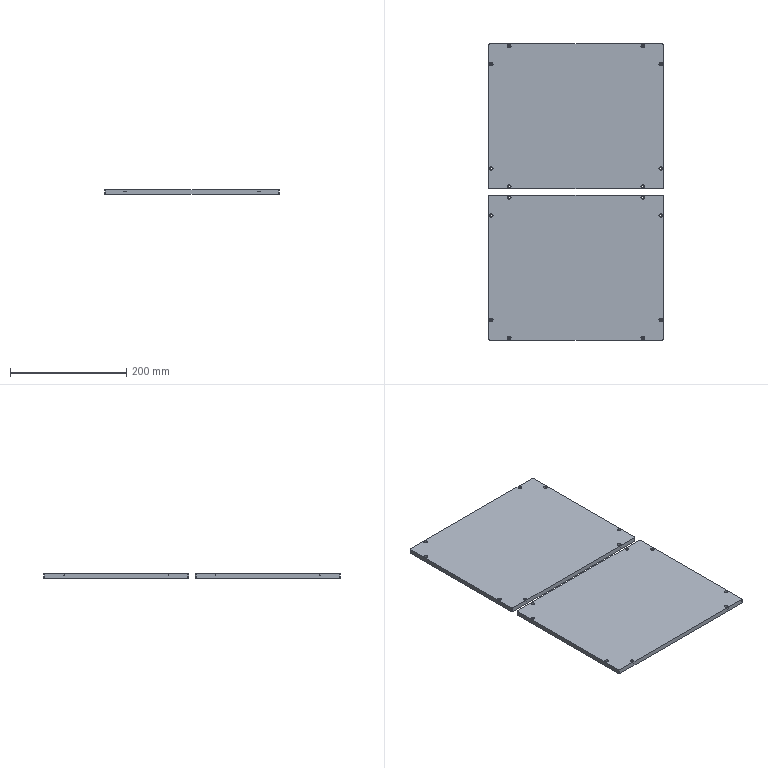NC program | NX | posted with a generic post | part box 300 x 511 x 8 mm
Whole program, first 1243 of 1446 lines:
N10 G17 G21 G94 G90
(ZLEVEL_PROFILE_1_COPY_1_COPY , TOOL : D4A45)
N12 T02 M6
N14 G54
N16 G17 G0 G90 X-219.556 Y146.806 S9500 M3
N18 G43 Z30. H2
N20 Z0.
N22 G94 G1 Z-1. F1000.
N24 X-220.154 Y147.841
N26 G3 X-220.5 Y148.041 R0.4
N28 X-222.541 Y146. R2.041
N30 X-220.5 Y148.041 R-2.041
N32 X-220.846 Y147.841 R0.4
N34 G1 X-221.444 Y146.806
N36 Z0.
N38 G0 Z30.
N40 Y-146.806
N42 Z0.
N44 G1 Z-1.
N46 X-220.846 Y-147.841
N48 G3 X-220.5 Y-148.041 R0.4
N50 G1 X-220.496
N52 G3 X-218.459 Y-145.996 R2.041
N54 X-220.5 Y-148.041 R-2.041
N56 X-220.154 Y-147.841 R0.4
N58 G1 X-219.556 Y-146.806
N60 Z0.
N62 G0 Z30.
N64 X-39.556 Y146.806
N66 Z0.
N68 G1 Z-1.
N70 X-40.154 Y147.841
N72 G3 X-40.5 Y148.041 R0.4
N74 G1 X-40.503
N76 G3 X-42.541 Y145.997 R2.041
N78 X-40.5 Y148.041 R-2.041
N80 X-40.846 Y147.841 R0.4
N82 G1 X-41.444 Y146.806
N84 Z0.
N86 G0 Z30.
N88 Y-146.806
N90 Z0.
N92 G1 Z-1.
N94 X-40.846 Y-147.841
N96 G3 X-40.5 Y-148.041 R0.4
N98 X-38.459 Y-146. R2.041
N100 X-40.5 Y-148.041 R-2.041
N102 X-40.154 Y-147.841 R0.4
N104 G1 X-39.556 Y-146.806
N106 Z0.
N108 G0 Z30.
N110 X-8.556 Y115.806
N112 Z0.
N114 G1 Z-1.
N116 X-9.154 Y116.841
N118 G3 X-9.5 Y117.041 R0.4
N120 G1 X-9.503
N122 G3 X-11.541 Y114.997 R2.041
N124 X-9.5 Y117.041 R-2.041
N126 X-9.846 Y116.841 R0.4
N128 G1 X-10.444 Y115.806
N130 Z0.
N132 G0 Z30.
N134 Y-115.806
N136 Z0.
N138 G1 Z-1.
N140 X-9.846 Y-116.841
N142 G3 X-9.5 Y-117.041 R0.4
N144 X-7.459 Y-115. R2.041
N146 X-9.5 Y-117.041 R-2.041
N148 X-9.154 Y-116.841 R0.4
N150 G1 X-8.556 Y-115.806
N152 Z0.
N154 G0 Z30.
N156 X-252.306 Y115.944
N158 Z0.
N160 G1 Z-1.
N162 X-253.341 Y115.346
N164 G3 X-253.541 Y115. R0.4
N166 X-251.5 Y112.959 R2.041
N168 X-253.541 Y115. R-2.041
N170 X-253.341 Y114.654 R0.4
N172 G1 X-252.306 Y114.056
N174 Z0.
N176 G0 Z30.
N178 Y-114.056
N180 Z0.
N182 G1 Z-1.
N184 X-253.341 Y-114.654
N186 G3 X-253.541 Y-115. R0.4
N188 X-251.5 Y-117.041 R2.041
N190 X-253.541 Y-115. R-2.041
N192 X-253.341 Y-115.346 R0.4
N194 G1 X-252.306 Y-115.944
N196 Z0.
N198 G0 Z30.
N200 X10.444 Y115.806
N202 Z0.
N204 G1 Z-1.
N206 X9.846 Y116.841
N208 G3 X9.5 Y117.041 R0.4
N210 X7.459 Y115. R2.041
N212 X9.5 Y117.041 R-2.041
N214 X9.154 Y116.841 R0.4
N216 G1 X8.556 Y115.806
N218 Z0.
N220 G0 Z30.
N222 Y-115.806
N224 Z0.
N226 G1 Z-1.
N228 X9.154 Y-116.841
N230 G3 X9.5 Y-117.041 R0.4
N232 G1 X9.502
N234 G3 X11.541 Y-114.998 R2.041
N236 X9.5 Y-117.041 R-2.041
N238 X9.846 Y-116.841 R0.4
N240 G1 X10.444 Y-115.806
N242 Z0.
N244 G0 Z30.
N246 X41.444 Y146.806
N248 Z0.
N250 G1 Z-1.
N252 X40.846 Y147.841
N254 G3 X40.5 Y148.041 R0.4
N256 X38.459 Y146. R2.041
N258 X40.5 Y148.041 R-2.041
N260 X40.154 Y147.841 R0.4
N262 G1 X39.556 Y146.806
N264 Z0.
N266 G0 Z30.
N268 Y-146.806
N270 Z0.
N272 G1 Z-1.
N274 X40.154 Y-147.841
N276 G3 X40.5 Y-148.041 R0.4
N278 G1 X40.503
N280 G3 X42.541 Y-145.997 R2.041
N282 X40.5 Y-148.041 R-2.041
N284 X40.846 Y-147.841 R0.4
N286 G1 X41.444 Y-146.806
N288 Z0.
N290 G0 Z30.
N292 X221.444 Y146.806
N294 Z0.
N296 G1 Z-1.
N298 X220.846 Y147.841
N300 G3 X220.5 Y148.041 R0.4
N302 G1 X220.496
N304 G3 X218.459 Y145.996 R2.041
N306 X220.5 Y148.041 R-2.041
N308 X220.154 Y147.841 R0.4
N310 G1 X219.556 Y146.806
N312 Z0.
N314 G0 Z30.
N316 Y-146.806
N318 Z0.
N320 G1 Z-1.
N322 X220.154 Y-147.841
N324 G3 X220.5 Y-148.041 R0.4
N326 X222.541 Y-146. R2.041
N328 X220.5 Y-148.041 R-2.041
N330 X220.846 Y-147.841 R0.4
N332 G1 X221.444 Y-146.806
N334 Z0.
N336 G0 Z30.
N338 X252.306 Y114.056
N340 Z0.
N342 G1 Z-1.
N344 X253.341 Y114.654
N346 G3 X253.541 Y115. R0.4
N348 X251.5 Y117.041 R2.041
N350 X253.541 Y115. R-2.041
N352 X253.341 Y115.346 R0.4
N354 G1 X252.306 Y115.944
N356 Z0.
N358 G0 Z30.
N360 Y-115.944
N362 Z0.
N364 G1 Z-1.
N366 X253.341 Y-115.346
N368 G3 X253.541 Y-115. R0.4
N370 X251.5 Y-112.959 R2.041
N372 X253.541 Y-115. R-2.041
N374 X253.341 Y-114.654 R0.4
N376 G1 X252.306 Y-114.056
N378 Z0.
N380 G0 Z30.
N382 X257.192 Y149.154
N384 Z0.
N386 G1 Z-1.
N388 X256.659 Y148.846
N390 G3 X256.459 Y148.5 R0.4
N392 G1 Y-148.5
N394 G2 X254. Y-150.959 R2.459
N396 G1 X7.
N398 G2 X4.541 Y-148.5 R2.459
N400 G1 Y148.5
N402 G2 X7. Y150.959 R2.459
N404 G1 X254.
N406 G2 X256.459 Y148.5 R2.459
N408 G3 X256.659 Y148.154 R0.4
N410 G1 X257.259 Y147.807
N412 Z0.
N414 G0 Z30.
N416 X-257.192 Y-149.154
N418 Z0.
N420 G1 Z-1.
N422 X-256.659 Y-148.846
N424 G3 X-256.459 Y-148.5 R0.4
N426 G1 Y148.5
N428 G2 X-254. Y150.959 R2.459
N430 G1 X-7.
N432 G2 X-4.541 Y148.5 R2.459
N434 G1 Y-148.5
N436 G2 X-7. Y-150.959 R2.459
N438 G1 X-254.
N440 G2 X-256.459 Y-148.5 R2.459
N442 G3 X-256.659 Y-148.154 R0.4
N444 G1 X-257.259 Y-147.807
N446 Z0.
N448 G0 Z30.
N450 M5
(HOLE_MILLING , TOOL : D4)
N452 T04 M6
N454 G54
N456 G17 G0 G90 X-251.5 Y115. S9500 M3
N458 G43 Z30. H4
N460 Z0.5
N462 G94 G3 X-251. Y115.5 R0.5 F1250.
N464 X-251.5 Y116. R0.5
N466 X-251.5 Y116. Z0.2 I0. J-1.
N468 X-251.5 Y116. Z-0.1 I0. J-1.
N470 X-251.5 Y116. Z-0.4 I0. J-1.
N472 X-251.5 Y116. Z-0.7 I0. J-1.
N474 X-251.5 Y116. Z-1. I0. J-1.
N476 X-251.5 Y116. Z-1.3 I0. J-1.
N478 X-251.5 Y116. Z-1.6 I0. J-1.
N480 X-251.5 Y116. Z-1.9 I0. J-1.
N482 X-251.5 Y116. Z-2.2 I0. J-1.
N484 X-251.5 Y116. Z-2.5 I0. J-1.
N486 X-251.5 Y116. Z-2.8 I0. J-1.
N488 X-251.5 Y116. Z-3.1 I0. J-1.
N490 X-251.5 Y116. Z-3.4 I0. J-1.
N492 X-252.366 Y114.5 Z-3.5 R1.
N494 X-251. Y114.134 R1.
N496 X-252.366 Y114.5 R-1.
N498 X-251.683 Y114.317 R0.5
N500 X-251.5 Y115. R0.5
N502 G0 Z30.
N504 X-220.5 Y146.
N506 Z0.5
N508 G3 X-220. Y146.5 R0.5
N510 X-220.5 Y147. R0.5
N512 X-220.5 Y147. Z0.2 I0. J-1.
N514 X-220.5 Y147. Z-0.1 I0. J-1.
N516 X-220.5 Y147. Z-0.4 I0. J-1.
N518 X-220.5 Y147. Z-0.7 I0. J-1.
N520 X-220.5 Y147. Z-1. I0. J-1.
N522 X-220.5 Y147. Z-1.3 I0. J-1.
N524 X-220.5 Y147. Z-1.6 I0. J-1.
N526 X-220.5 Y147. Z-1.9 I0. J-1.
N528 X-220.5 Y147. Z-2.2 I0. J-1.
N530 X-220.5 Y147. Z-2.5 I0. J-1.
N532 X-220.5 Y147. Z-2.8 I0. J-1.
N534 X-220.5 Y147. Z-3.1 I0. J-1.
N536 X-220.5 Y147. Z-3.4 I0. J-1.
N538 X-221.366 Y145.5 Z-3.5 R1.
N540 X-220. Y145.134 R1.
N542 X-221.366 Y145.5 R-1.
N544 X-220.683 Y145.317 R0.5
N546 X-220.5 Y146. R0.5
N548 G0 Z30.
N550 X-40.5
N552 Z0.5
N554 G3 X-40. Y146.5 R0.5
N556 X-40.5 Y147. R0.5
N558 X-40.5 Y147. Z0.2 I0. J-1.
N560 X-40.5 Y147. Z-0.1 I0. J-1.
N562 X-40.5 Y147. Z-0.4 I0. J-1.
N564 X-40.5 Y147. Z-0.7 I0. J-1.
N566 X-40.5 Y147. Z-1. I0. J-1.
N568 X-40.5 Y147. Z-1.3 I0. J-1.
N570 X-40.5 Y147. Z-1.6 I0. J-1.
N572 X-40.5 Y147. Z-1.9 I0. J-1.
N574 X-40.5 Y147. Z-2.2 I0. J-1.
N576 X-40.5 Y147. Z-2.5 I0. J-1.
N578 X-40.5 Y147. Z-2.8 I0. J-1.
N580 X-40.5 Y147. Z-3.1 I0. J-1.
N582 X-40.5 Y147. Z-3.4 I0. J-1.
N584 X-41.366 Y145.5 Z-3.5 R1.
N586 X-40. Y145.134 R1.
N588 X-41.366 Y145.5 R-1.
N590 X-40.683 Y145.317 R0.5
N592 X-40.5 Y146. R0.5
N594 G0 Z30.
N596 X-9.5 Y115.
N598 Z0.5
N600 G3 X-9. Y115.5 R0.5
N602 X-9.5 Y116. R0.5
N604 X-9.5 Y116. Z0.2 I0. J-1.
N606 X-9.5 Y116. Z-0.1 I0. J-1.
N608 X-9.5 Y116. Z-0.4 I0. J-1.
N610 X-9.5 Y116. Z-0.7 I0. J-1.
N612 X-9.5 Y116. Z-1. I0. J-1.
N614 X-9.5 Y116. Z-1.3 I0. J-1.
N616 X-9.5 Y116. Z-1.6 I0. J-1.
N618 X-9.5 Y116. Z-1.9 I0. J-1.
N620 X-9.5 Y116. Z-2.2 I0. J-1.
N622 X-9.5 Y116. Z-2.5 I0. J-1.
N624 X-9.5 Y116. Z-2.8 I0. J-1.
N626 X-9.5 Y116. Z-3.1 I0. J-1.
N628 X-9.5 Y116. Z-3.4 I0. J-1.
N630 X-10.366 Y114.5 Z-3.5 R1.
N632 X-9. Y114.134 R1.
N634 X-10.366 Y114.5 R-1.
N636 X-9.683 Y114.317 R0.5
N638 X-9.5 Y115. R0.5
N640 G0 Z30.
N642 X9.5
N644 Z0.5
N646 G3 X10. Y115.5 R0.5
N648 X9.5 Y116. R0.5
N650 X9.5 Y116. Z0.2 I0. J-1.
N652 X9.5 Y116. Z-0.1 I0. J-1.
N654 X9.5 Y116. Z-0.4 I0. J-1.
N656 X9.5 Y116. Z-0.7 I0. J-1.
N658 X9.5 Y116. Z-1. I0. J-1.
N660 X9.5 Y116. Z-1.3 I0. J-1.
N662 X9.5 Y116. Z-1.6 I0. J-1.
N664 X9.5 Y116. Z-1.9 I0. J-1.
N666 X9.5 Y116. Z-2.2 I0. J-1.
N668 X9.5 Y116. Z-2.5 I0. J-1.
N670 X9.5 Y116. Z-2.8 I0. J-1.
N672 X9.5 Y116. Z-3.1 I0. J-1.
N674 X9.5 Y116. Z-3.4 I0. J-1.
N676 X8.634 Y114.5 Z-3.5 R1.
N678 X10. Y114.134 R1.
N680 X8.634 Y114.5 R-1.
N682 X9.317 Y114.317 R0.5
N684 X9.5 Y115. R0.5
N686 G0 Z30.
N688 X40.5 Y146.
N690 Z0.5
N692 G3 X41. Y146.5 R0.5
N694 X40.5 Y147. R0.5
N696 X40.5 Y147. Z0.2 I0. J-1.
N698 X40.5 Y147. Z-0.1 I0. J-1.
N700 X40.5 Y147. Z-0.4 I0. J-1.
N702 X40.5 Y147. Z-0.7 I0. J-1.
N704 X40.5 Y147. Z-1. I0. J-1.
N706 X40.5 Y147. Z-1.3 I0. J-1.
N708 X40.5 Y147. Z-1.6 I0. J-1.
N710 X40.5 Y147. Z-1.9 I0. J-1.
N712 X40.5 Y147. Z-2.2 I0. J-1.
N714 X40.5 Y147. Z-2.5 I0. J-1.
N716 X40.5 Y147. Z-2.8 I0. J-1.
N718 X40.5 Y147. Z-3.1 I0. J-1.
N720 X40.5 Y147. Z-3.4 I0. J-1.
N722 X39.634 Y145.5 Z-3.5 R1.
N724 X41. Y145.134 R1.
N726 X39.634 Y145.5 R-1.
N728 X40.317 Y145.317 R0.5
N730 X40.5 Y146. R0.5
N732 G0 Z30.
N734 X220.5
N736 Z0.5
N738 G3 X221. Y146.5 R0.5
N740 X220.5 Y147. R0.5
N742 X220.5 Y147. Z0.2 I0. J-1.
N744 X220.5 Y147. Z-0.1 I0. J-1.
N746 X220.5 Y147. Z-0.4 I0. J-1.
N748 X220.5 Y147. Z-0.7 I0. J-1.
N750 X220.5 Y147. Z-1. I0. J-1.
N752 X220.5 Y147. Z-1.3 I0. J-1.
N754 X220.5 Y147. Z-1.6 I0. J-1.
N756 X220.5 Y147. Z-1.9 I0. J-1.
N758 X220.5 Y147. Z-2.2 I0. J-1.
N760 X220.5 Y147. Z-2.5 I0. J-1.
N762 X220.5 Y147. Z-2.8 I0. J-1.
N764 X220.5 Y147. Z-3.1 I0. J-1.
N766 X220.5 Y147. Z-3.4 I0. J-1.
N768 X219.634 Y145.5 Z-3.5 R1.
N770 X221. Y145.134 R1.
N772 X219.634 Y145.5 R-1.
N774 X220.317 Y145.317 R0.5
N776 X220.5 Y146. R0.5
N778 G0 Z30.
N780 X251.5 Y115.
N782 Z0.5
N784 G3 X252. Y115.5 R0.5
N786 X251.5 Y116. R0.5
N788 X251.5 Y116. Z0.2 I0. J-1.
N790 X251.5 Y116. Z-0.1 I0. J-1.
N792 X251.5 Y116. Z-0.4 I0. J-1.
N794 X251.5 Y116. Z-0.7 I0. J-1.
N796 X251.5 Y116. Z-1. I0. J-1.
N798 X251.5 Y116. Z-1.3 I0. J-1.
N800 X251.5 Y116. Z-1.6 I0. J-1.
N802 X251.5 Y116. Z-1.9 I0. J-1.
N804 X251.5 Y116. Z-2.2 I0. J-1.
N806 X251.5 Y116. Z-2.5 I0. J-1.
N808 X251.5 Y116. Z-2.8 I0. J-1.
N810 X251.5 Y116. Z-3.1 I0. J-1.
N812 X251.5 Y116. Z-3.4 I0. J-1.
N814 X250.634 Y114.5 Z-3.5 R1.
N816 X252. Y114.134 R1.
N818 X250.634 Y114.5 R-1.
N820 X251.317 Y114.317 R0.5
N822 X251.5 Y115. R0.5
N824 G0 Z30.
N826 Y-115.
N828 Z0.5
N830 G3 X252. Y-114.5 R0.5
N832 X251.5 Y-114. R0.5
N834 X251.5 Y-114. Z0.2 I0. J-1.
N836 X251.5 Y-114. Z-0.1 I0. J-1.
N838 X251.5 Y-114. Z-0.4 I0. J-1.
N840 X251.5 Y-114. Z-0.7 I0. J-1.
N842 X251.5 Y-114. Z-1. I0. J-1.
N844 X251.5 Y-114. Z-1.3 I0. J-1.
N846 X251.5 Y-114. Z-1.6 I0. J-1.
N848 X251.5 Y-114. Z-1.9 I0. J-1.
N850 X251.5 Y-114. Z-2.2 I0. J-1.
N852 X251.5 Y-114. Z-2.5 I0. J-1.
N854 X251.5 Y-114. Z-2.8 I0. J-1.
N856 X251.5 Y-114. Z-3.1 I0. J-1.
N858 X251.5 Y-114. Z-3.4 I0. J-1.
N860 X250.634 Y-115.5 Z-3.5 R1.
N862 X252. Y-115.866 R1.
N864 X250.634 Y-115.5 R-1.
N866 X251.317 Y-115.683 R0.5
N868 X251.5 Y-115. R0.5
N870 G0 Z30.
N872 X220.5 Y-146.
N874 Z0.5
N876 G3 X221. Y-145.5 R0.5
N878 X220.5 Y-145. R0.5
N880 X220.5 Y-145. Z0.2 I0. J-1.
N882 X220.5 Y-145. Z-0.1 I0. J-1.
N884 X220.5 Y-145. Z-0.4 I0. J-1.
N886 X220.5 Y-145. Z-0.7 I0. J-1.
N888 X220.5 Y-145. Z-1. I0. J-1.
N890 X220.5 Y-145. Z-1.3 I0. J-1.
N892 X220.5 Y-145. Z-1.6 I0. J-1.
N894 X220.5 Y-145. Z-1.9 I0. J-1.
N896 X220.5 Y-145. Z-2.2 I0. J-1.
N898 X220.5 Y-145. Z-2.5 I0. J-1.
N900 X220.5 Y-145. Z-2.8 I0. J-1.
N902 X220.5 Y-145. Z-3.1 I0. J-1.
N904 X220.5 Y-145. Z-3.4 I0. J-1.
N906 X219.634 Y-146.5 Z-3.5 R1.
N908 X221. Y-146.866 R1.
N910 X219.634 Y-146.5 R-1.
N912 X220.317 Y-146.683 R0.5
N914 X220.5 Y-146. R0.5
N916 G0 Z30.
N918 X40.5
N920 Z0.5
N922 G3 X41. Y-145.5 R0.5
N924 X40.5 Y-145. R0.5
N926 X40.5 Y-145. Z0.2 I0. J-1.
N928 X40.5 Y-145. Z-0.1 I0. J-1.
N930 X40.5 Y-145. Z-0.4 I0. J-1.
N932 X40.5 Y-145. Z-0.7 I0. J-1.
N934 X40.5 Y-145. Z-1. I0. J-1.
N936 X40.5 Y-145. Z-1.3 I0. J-1.
N938 X40.5 Y-145. Z-1.6 I0. J-1.
N940 X40.5 Y-145. Z-1.9 I0. J-1.
N942 X40.5 Y-145. Z-2.2 I0. J-1.
N944 X40.5 Y-145. Z-2.5 I0. J-1.
N946 X40.5 Y-145. Z-2.8 I0. J-1.
N948 X40.5 Y-145. Z-3.1 I0. J-1.
N950 X40.5 Y-145. Z-3.4 I0. J-1.
N952 X39.634 Y-146.5 Z-3.5 R1.
N954 X41. Y-146.866 R1.
N956 X39.634 Y-146.5 R-1.
N958 X40.317 Y-146.683 R0.5
N960 X40.5 Y-146. R0.5
N962 G0 Z30.
N964 X9.5 Y-115.
N966 Z0.5
N968 G3 X10. Y-114.5 R0.5
N970 X9.5 Y-114. R0.5
N972 X9.5 Y-114. Z0.2 I0. J-1.
N974 X9.5 Y-114. Z-0.1 I0. J-1.
N976 X9.5 Y-114. Z-0.4 I0. J-1.
N978 X9.5 Y-114. Z-0.7 I0. J-1.
N980 X9.5 Y-114. Z-1. I0. J-1.
N982 X9.5 Y-114. Z-1.3 I0. J-1.
N984 X9.5 Y-114. Z-1.6 I0. J-1.
N986 X9.5 Y-114. Z-1.9 I0. J-1.
N988 X9.5 Y-114. Z-2.2 I0. J-1.
N990 X9.5 Y-114. Z-2.5 I0. J-1.
N992 X9.5 Y-114. Z-2.8 I0. J-1.
N994 X9.5 Y-114. Z-3.1 I0. J-1.
N996 X9.5 Y-114. Z-3.4 I0. J-1.
N998 X8.634 Y-115.5 Z-3.5 R1.
N1000 X10. Y-115.866 R1.
N1002 X8.634 Y-115.5 R-1.
N1004 X9.317 Y-115.683 R0.5
N1006 X9.5 Y-115. R0.5
N1008 G0 Z30.
N1010 X-9.5
N1012 Z0.5
N1014 G3 X-9. Y-114.5 R0.5
N1016 X-9.5 Y-114. R0.5
N1018 X-9.5 Y-114. Z0.2 I0. J-1.
N1020 X-9.5 Y-114. Z-0.1 I0. J-1.
N1022 X-9.5 Y-114. Z-0.4 I0. J-1.
N1024 X-9.5 Y-114. Z-0.7 I0. J-1.
N1026 X-9.5 Y-114. Z-1. I0. J-1.
N1028 X-9.5 Y-114. Z-1.3 I0. J-1.
N1030 X-9.5 Y-114. Z-1.6 I0. J-1.
N1032 X-9.5 Y-114. Z-1.9 I0. J-1.
N1034 X-9.5 Y-114. Z-2.2 I0. J-1.
N1036 X-9.5 Y-114. Z-2.5 I0. J-1.
N1038 X-9.5 Y-114. Z-2.8 I0. J-1.
N1040 X-9.5 Y-114. Z-3.1 I0. J-1.
N1042 X-9.5 Y-114. Z-3.4 I0. J-1.
N1044 X-10.366 Y-115.5 Z-3.5 R1.
N1046 X-9. Y-115.866 R1.
N1048 X-10.366 Y-115.5 R-1.
N1050 X-9.683 Y-115.683 R0.5
N1052 X-9.5 Y-115. R0.5
N1054 G0 Z30.
N1056 X-40.5 Y-146.
N1058 Z0.5
N1060 G3 X-40. Y-145.5 R0.5
N1062 X-40.5 Y-145. R0.5
N1064 X-40.5 Y-145. Z0.2 I0. J-1.
N1066 X-40.5 Y-145. Z-0.1 I0. J-1.
N1068 X-40.5 Y-145. Z-0.4 I0. J-1.
N1070 X-40.5 Y-145. Z-0.7 I0. J-1.
N1072 X-40.5 Y-145. Z-1. I0. J-1.
N1074 X-40.5 Y-145. Z-1.3 I0. J-1.
N1076 X-40.5 Y-145. Z-1.6 I0. J-1.
N1078 X-40.5 Y-145. Z-1.9 I0. J-1.
N1080 X-40.5 Y-145. Z-2.2 I0. J-1.
N1082 X-40.5 Y-145. Z-2.5 I0. J-1.
N1084 X-40.5 Y-145. Z-2.8 I0. J-1.
N1086 X-40.5 Y-145. Z-3.1 I0. J-1.
N1088 X-40.5 Y-145. Z-3.4 I0. J-1.
N1090 X-41.366 Y-146.5 Z-3.5 R1.
N1092 X-40. Y-146.866 R1.
N1094 X-41.366 Y-146.5 R-1.
N1096 X-40.683 Y-146.683 R0.5
N1098 X-40.5 Y-146. R0.5
N1100 G0 Z30.
N1102 X-220.5
N1104 Z0.5
N1106 G3 X-220. Y-145.5 R0.5
N1108 X-220.5 Y-145. R0.5
N1110 X-220.5 Y-145. Z0.2 I0. J-1.
N1112 X-220.5 Y-145. Z-0.1 I0. J-1.
N1114 X-220.5 Y-145. Z-0.4 I0. J-1.
N1116 X-220.5 Y-145. Z-0.7 I0. J-1.
N1118 X-220.5 Y-145. Z-1. I0. J-1.
N1120 X-220.5 Y-145. Z-1.3 I0. J-1.
N1122 X-220.5 Y-145. Z-1.6 I0. J-1.
N1124 X-220.5 Y-145. Z-1.9 I0. J-1.
N1126 X-220.5 Y-145. Z-2.2 I0. J-1.
N1128 X-220.5 Y-145. Z-2.5 I0. J-1.
N1130 X-220.5 Y-145. Z-2.8 I0. J-1.
N1132 X-220.5 Y-145. Z-3.1 I0. J-1.
N1134 X-220.5 Y-145. Z-3.4 I0. J-1.
N1136 X-221.366 Y-146.5 Z-3.5 R1.
N1138 X-220. Y-146.866 R1.
N1140 X-221.366 Y-146.5 R-1.
N1142 X-220.683 Y-146.683 R0.5
N1144 X-220.5 Y-146. R0.5
N1146 G0 Z30.
N1148 X-251.5 Y-115.
N1150 Z0.5
N1152 G3 X-251. Y-114.5 R0.5
N1154 X-251.5 Y-114. R0.5
N1156 X-251.5 Y-114. Z0.2 I0. J-1.
N1158 X-251.5 Y-114. Z-0.1 I0. J-1.
N1160 X-251.5 Y-114. Z-0.4 I0. J-1.
N1162 X-251.5 Y-114. Z-0.7 I0. J-1.
N1164 X-251.5 Y-114. Z-1. I0. J-1.
N1166 X-251.5 Y-114. Z-1.3 I0. J-1.
N1168 X-251.5 Y-114. Z-1.6 I0. J-1.
N1170 X-251.5 Y-114. Z-1.9 I0. J-1.
N1172 X-251.5 Y-114. Z-2.2 I0. J-1.
N1174 X-251.5 Y-114. Z-2.5 I0. J-1.
N1176 X-251.5 Y-114. Z-2.8 I0. J-1.
N1178 X-251.5 Y-114. Z-3.1 I0. J-1.
N1180 X-251.5 Y-114. Z-3.4 I0. J-1.
N1182 X-252.366 Y-115.5 Z-3.5 R1.
N1184 X-251. Y-115.866 R1.
N1186 X-252.366 Y-115.5 R-1.
N1188 X-251.683 Y-115.683 R0.5
N1190 X-251.5 Y-115. R0.5
N1192 G0 Z30.
N1194 M5
(HOLE_MILLING_COPY , TOOL : D2)
N1196 T12 M6
N1198 G54
N1200 G17 G0 G90 X-251.5 Y115. S9500 M3
N1202 G43 Z30. H12
N1204 Z-3.
N1206 G94 G3 X-251.125 Y115.375 R0.375 F1100.
N1208 X-251.5 Y115.75 R0.375
N1210 X-251.5 Y115.75 Z-3.15 I0. J-0.75
N1212 X-251.5 Y115.75 Z-3.3 I0. J-0.75
N1214 X-251.5 Y115.75 Z-3.45 I0. J-0.75
N1216 X-251.5 Y115.75 Z-3.6 I0. J-0.75
N1218 X-251.5 Y115.75 Z-3.75 I0. J-0.75
N1220 X-251.5 Y115.75 Z-3.9 I0. J-0.75
N1222 X-251.5 Y115.75 Z-4.05 I0. J-0.75
N1224 X-251.5 Y115.75 Z-4.2 I0. J-0.75
N1226 X-251.5 Y115.75 Z-4.35 I0. J-0.75
N1228 X-251.5 Y115.75 Z-4.5 I0. J-0.75
N1230 X-251.5 Y115.75 Z-4.65 I0. J-0.75
N1232 X-251.5 Y115.75 Z-4.8 I0. J-0.75
N1234 X-251.5 Y115.75 Z-4.95 I0. J-0.75
N1236 X-251.5 Y115.75 Z-5.1 I0. J-0.75
N1238 X-251.5 Y115.75 Z-5.25 I0. J-0.75
N1240 X-251.5 Y115.75 Z-5.4 I0. J-0.75
N1242 X-251.5 Y115.75 Z-5.55 I0. J-0.75
N1244 X-251.5 Y115.75 Z-5.7 I0. J-0.75
N1246 X-251.5 Y115.75 Z-5.85 I0. J-0.75
N1248 X-251.5 Y115.75 Z-6. I0. J-0.75
N1250 X-251.5 Y115.75 Z-6.15 I0. J-0.75
N1252 X-251.5 Y115.75 Z-6.3 I0. J-0.75
N1254 X-251.5 Y115.75 Z-6.45 I0. J-0.75
N1256 X-251.5 Y115.75 Z-6.6 I0. J-0.75
N1258 X-251.5 Y115.75 Z-6.75 I0. J-0.75
N1260 X-251.5 Y115.75 Z-6.9 I0. J-0.75
N1262 X-251.5 Y115.75 Z-7.05 I0. J-0.75
N1264 X-251.5 Y115.75 Z-7.2 I0. J-0.75
N1266 X-251.5 Y115.75 Z-7.35 I0. J-0.75
N1268 X-251.5 Y115.75 Z-7.5 I0. J-0.75
N1270 X-251.5 Y115.75 Z-7.65 I0. J-0.75
N1272 X-251.5 Y115.75 Z-7.8 I0. J-0.75
N1274 X-252.15 Y114.625 Z-7.85 R0.75
N1276 X-251.125 Y114.35 R0.75
N1278 X-252.15 Y114.625 R-0.75
N1280 X-251.637 Y114.488 R0.375
N1282 X-251.5 Y115. R0.375
N1284 G0 Z30.
N1286 X-220.5 Y146.
N1288 Z-3.
N1290 G3 X-220.125 Y146.375 R0.375
N1292 X-220.5 Y146.75 R0.375
N1294 X-220.5 Y146.75 Z-3.15 I0. J-0.75
N1296 X-220.5 Y146.75 Z-3.3 I0. J-0.75
N1298 X-220.5 Y146.75 Z-3.45 I0. J-0.75
N1300 X-220.5 Y146.75 Z-3.6 I0. J-0.75
N1302 X-220.5 Y146.75 Z-3.75 I0. J-0.75
N1304 X-220.5 Y146.75 Z-3.9 I0. J-0.75
N1306 X-220.5 Y146.75 Z-4.05 I0. J-0.75
N1308 X-220.5 Y146.75 Z-4.2 I0. J-0.75
N1310 X-220.5 Y146.75 Z-4.35 I0. J-0.75
N1312 X-220.5 Y146.75 Z-4.5 I0. J-0.75
N1314 X-220.5 Y146.75 Z-4.65 I0. J-0.75
N1316 X-220.5 Y146.75 Z-4.8 I0. J-0.75
N1318 X-220.5 Y146.75 Z-4.95 I0. J-0.75
N1320 X-220.5 Y146.75 Z-5.1 I0. J-0.75
N1322 X-220.5 Y146.75 Z-5.25 I0. J-0.75
N1324 X-220.5 Y146.75 Z-5.4 I0. J-0.75
N1326 X-220.5 Y146.75 Z-5.55 I0. J-0.75
N1328 X-220.5 Y146.75 Z-5.7 I0. J-0.75
N1330 X-220.5 Y146.75 Z-5.85 I0. J-0.75
N1332 X-220.5 Y146.75 Z-6. I0. J-0.75
N1334 X-220.5 Y146.75 Z-6.15 I0. J-0.75
N1336 X-220.5 Y146.75 Z-6.3 I0. J-0.75
N1338 X-220.5 Y146.75 Z-6.45 I0. J-0.75
N1340 X-220.5 Y146.75 Z-6.6 I0. J-0.75
N1342 X-220.5 Y146.75 Z-6.75 I0. J-0.75
N1344 X-220.5 Y146.75 Z-6.9 I0. J-0.75
N1346 X-220.5 Y146.75 Z-7.05 I0. J-0.75
N1348 X-220.5 Y146.75 Z-7.2 I0. J-0.75
N1350 X-220.5 Y146.75 Z-7.35 I0. J-0.75
N1352 X-220.5 Y146.75 Z-7.5 I0. J-0.75
N1354 X-220.5 Y146.75 Z-7.65 I0. J-0.75
N1356 X-220.5 Y146.75 Z-7.8 I0. J-0.75
N1358 X-221.15 Y145.625 Z-7.85 R0.75
N1360 X-220.125 Y145.35 R0.75
N1362 X-221.15 Y145.625 R-0.75
N1364 X-220.637 Y145.488 R0.375
N1366 X-220.5 Y146. R0.375
N1368 G0 Z30.
N1370 X-40.5
N1372 Z-3.
N1374 G3 X-40.125 Y146.375 R0.375
N1376 X-40.5 Y146.75 R0.375
N1378 X-40.5 Y146.75 Z-3.15 I0. J-0.75
N1380 X-40.5 Y146.75 Z-3.3 I0. J-0.75
N1382 X-40.5 Y146.75 Z-3.45 I0. J-0.75
N1384 X-40.5 Y146.75 Z-3.6 I0. J-0.75
N1386 X-40.5 Y146.75 Z-3.75 I0. J-0.75
N1388 X-40.5 Y146.75 Z-3.9 I0. J-0.75
N1390 X-40.5 Y146.75 Z-4.05 I0. J-0.75
N1392 X-40.5 Y146.75 Z-4.2 I0. J-0.75
N1394 X-40.5 Y146.75 Z-4.35 I0. J-0.75
N1396 X-40.5 Y146.75 Z-4.5 I0. J-0.75
N1398 X-40.5 Y146.75 Z-4.65 I0. J-0.75
N1400 X-40.5 Y146.75 Z-4.8 I0. J-0.75
N1402 X-40.5 Y146.75 Z-4.95 I0. J-0.75
N1404 X-40.5 Y146.75 Z-5.1 I0. J-0.75
N1406 X-40.5 Y146.75 Z-5.25 I0. J-0.75
N1408 X-40.5 Y146.75 Z-5.4 I0. J-0.75
N1410 X-40.5 Y146.75 Z-5.55 I0. J-0.75
N1412 X-40.5 Y146.75 Z-5.7 I0. J-0.75
N1414 X-40.5 Y146.75 Z-5.85 I0. J-0.75
N1416 X-40.5 Y146.75 Z-6. I0. J-0.75
N1418 X-40.5 Y146.75 Z-6.15 I0. J-0.75
N1420 X-40.5 Y146.75 Z-6.3 I0. J-0.75
N1422 X-40.5 Y146.75 Z-6.45 I0. J-0.75
N1424 X-40.5 Y146.75 Z-6.6 I0. J-0.75
N1426 X-40.5 Y146.75 Z-6.75 I0. J-0.75
N1428 X-40.5 Y146.75 Z-6.9 I0. J-0.75
N1430 X-40.5 Y146.75 Z-7.05 I0. J-0.75
N1432 X-40.5 Y146.75 Z-7.2 I0. J-0.75
N1434 X-40.5 Y146.75 Z-7.35 I0. J-0.75
N1436 X-40.5 Y146.75 Z-7.5 I0. J-0.75
N1438 X-40.5 Y146.75 Z-7.65 I0. J-0.75
N1440 X-40.5 Y146.75 Z-7.8 I0. J-0.75
N1442 X-41.15 Y145.625 Z-7.85 R0.75
N1444 X-40.125 Y145.35 R0.75
N1446 X-41.15 Y145.625 R-0.75
N1448 X-40.637 Y145.488 R0.375
N1450 X-40.5 Y146. R0.375
N1452 G0 Z30.
N1454 X-9.5 Y115.
N1456 Z-3.
N1458 G3 X-9.125 Y115.375 R0.375
N1460 X-9.5 Y115.75 R0.375
N1462 X-9.5 Y115.75 Z-3.15 I0. J-0.75
N1464 X-9.5 Y115.75 Z-3.3 I0. J-0.75
N1466 X-9.5 Y115.75 Z-3.45 I0. J-0.75
N1468 X-9.5 Y115.75 Z-3.6 I0. J-0.75
N1470 X-9.5 Y115.75 Z-3.75 I0. J-0.75
N1472 X-9.5 Y115.75 Z-3.9 I0. J-0.75
N1474 X-9.5 Y115.75 Z-4.05 I0. J-0.75
N1476 X-9.5 Y115.75 Z-4.2 I0. J-0.75
N1478 X-9.5 Y115.75 Z-4.35 I0. J-0.75
N1480 X-9.5 Y115.75 Z-4.5 I0. J-0.75
N1482 X-9.5 Y115.75 Z-4.65 I0. J-0.75
N1484 X-9.5 Y115.75 Z-4.8 I0. J-0.75
N1486 X-9.5 Y115.75 Z-4.95 I0. J-0.75
N1488 X-9.5 Y115.75 Z-5.1 I0. J-0.75
N1490 X-9.5 Y115.75 Z-5.25 I0. J-0.75
N1492 X-9.5 Y115.75 Z-5.4 I0. J-0.75
N1494 X-9.5 Y115.75 Z-5.55 I0. J-0.75
N1496 X-9.5 Y115.75 Z-5.7 I0. J-0.75
N1498 X-9.5 Y115.75 Z-5.85 I0. J-0.75
N1500 X-9.5 Y115.75 Z-6. I0. J-0.75
N1502 X-9.5 Y115.75 Z-6.15 I0. J-0.75
N1504 X-9.5 Y115.75 Z-6.3 I0. J-0.75
N1506 X-9.5 Y115.75 Z-6.45 I0. J-0.75
N1508 X-9.5 Y115.75 Z-6.6 I0. J-0.75
N1510 X-9.5 Y115.75 Z-6.75 I0. J-0.75
N1512 X-9.5 Y115.75 Z-6.9 I0. J-0.75
N1514 X-9.5 Y115.75 Z-7.05 I0. J-0.75
N1516 X-9.5 Y115.75 Z-7.2 I0. J-0.75
N1518 X-9.5 Y115.75 Z-7.35 I0. J-0.75
N1520 X-9.5 Y115.75 Z-7.5 I0. J-0.75
N1522 X-9.5 Y115.75 Z-7.65 I0. J-0.75
N1524 X-9.5 Y115.75 Z-7.8 I0. J-0.75
N1526 X-10.15 Y114.625 Z-7.85 R0.75
N1528 X-9.125 Y114.35 R0.75
N1530 X-10.15 Y114.625 R-0.75
N1532 X-9.637 Y114.488 R0.375
N1534 X-9.5 Y115. R0.375
N1536 G0 Z30.
N1538 X9.5
N1540 Z-3.
N1542 G3 X9.875 Y115.375 R0.375
N1544 X9.5 Y115.75 R0.375
N1546 X9.5 Y115.75 Z-3.15 I0. J-0.75
N1548 X9.5 Y115.75 Z-3.3 I0. J-0.75
N1550 X9.5 Y115.75 Z-3.45 I0. J-0.75
N1552 X9.5 Y115.75 Z-3.6 I0. J-0.75
N1554 X9.5 Y115.75 Z-3.75 I0. J-0.75
N1556 X9.5 Y115.75 Z-3.9 I0. J-0.75
N1558 X9.5 Y115.75 Z-4.05 I0. J-0.75
N1560 X9.5 Y115.75 Z-4.2 I0. J-0.75
N1562 X9.5 Y115.75 Z-4.35 I0. J-0.75
N1564 X9.5 Y115.75 Z-4.5 I0. J-0.75
N1566 X9.5 Y115.75 Z-4.65 I0. J-0.75
N1568 X9.5 Y115.75 Z-4.8 I0. J-0.75
N1570 X9.5 Y115.75 Z-4.95 I0. J-0.75
N1572 X9.5 Y115.75 Z-5.1 I0. J-0.75
N1574 X9.5 Y115.75 Z-5.25 I0. J-0.75
N1576 X9.5 Y115.75 Z-5.4 I0. J-0.75
N1578 X9.5 Y115.75 Z-5.55 I0. J-0.75
N1580 X9.5 Y115.75 Z-5.7 I0. J-0.75
N1582 X9.5 Y115.75 Z-5.85 I0. J-0.75
N1584 X9.5 Y115.75 Z-6. I0. J-0.75
N1586 X9.5 Y115.75 Z-6.15 I0. J-0.75
N1588 X9.5 Y115.75 Z-6.3 I0. J-0.75
N1590 X9.5 Y115.75 Z-6.45 I0. J-0.75
N1592 X9.5 Y115.75 Z-6.6 I0. J-0.75
N1594 X9.5 Y115.75 Z-6.75 I0. J-0.75
N1596 X9.5 Y115.75 Z-6.9 I0. J-0.75
N1598 X9.5 Y115.75 Z-7.05 I0. J-0.75
N1600 X9.5 Y115.75 Z-7.2 I0. J-0.75
N1602 X9.5 Y115.75 Z-7.35 I0. J-0.75
N1604 X9.5 Y115.75 Z-7.5 I0. J-0.75
N1606 X9.5 Y115.75 Z-7.65 I0. J-0.75
N1608 X9.5 Y115.75 Z-7.8 I0. J-0.75
N1610 X8.85 Y114.625 Z-7.85 R0.75
N1612 X9.875 Y114.35 R0.75
N1614 X8.85 Y114.625 R-0.75
N1616 X9.363 Y114.488 R0.375
N1618 X9.5 Y115. R0.375
N1620 G0 Z30.
N1622 X40.5 Y146.
N1624 Z-3.
N1626 G3 X40.875 Y146.375 R0.375
N1628 X40.5 Y146.75 R0.375
N1630 X40.5 Y146.75 Z-3.15 I0. J-0.75
N1632 X40.5 Y146.75 Z-3.3 I0. J-0.75
N1634 X40.5 Y146.75 Z-3.45 I0. J-0.75
N1636 X40.5 Y146.75 Z-3.6 I0. J-0.75
N1638 X40.5 Y146.75 Z-3.75 I0. J-0.75
N1640 X40.5 Y146.75 Z-3.9 I0. J-0.75
N1642 X40.5 Y146.75 Z-4.05 I0. J-0.75
N1644 X40.5 Y146.75 Z-4.2 I0. J-0.75
N1646 X40.5 Y146.75 Z-4.35 I0. J-0.75
N1648 X40.5 Y146.75 Z-4.5 I0. J-0.75
N1650 X40.5 Y146.75 Z-4.65 I0. J-0.75
N1652 X40.5 Y146.75 Z-4.8 I0. J-0.75
N1654 X40.5 Y146.75 Z-4.95 I0. J-0.75
N1656 X40.5 Y146.75 Z-5.1 I0. J-0.75
N1658 X40.5 Y146.75 Z-5.25 I0. J-0.75
N1660 X40.5 Y146.75 Z-5.4 I0. J-0.75
N1662 X40.5 Y146.75 Z-5.55 I0. J-0.75
N1664 X40.5 Y146.75 Z-5.7 I0. J-0.75
N1666 X40.5 Y146.75 Z-5.85 I0. J-0.75
N1668 X40.5 Y146.75 Z-6. I0. J-0.75
N1670 X40.5 Y146.75 Z-6.15 I0. J-0.75
N1672 X40.5 Y146.75 Z-6.3 I0. J-0.75
N1674 X40.5 Y146.75 Z-6.45 I0. J-0.75
N1676 X40.5 Y146.75 Z-6.6 I0. J-0.75
N1678 X40.5 Y146.75 Z-6.75 I0. J-0.75
N1680 X40.5 Y146.75 Z-6.9 I0. J-0.75
N1682 X40.5 Y146.75 Z-7.05 I0. J-0.75
N1684 X40.5 Y146.75 Z-7.2 I0. J-0.75
N1686 X40.5 Y146.75 Z-7.35 I0. J-0.75
N1688 X40.5 Y146.75 Z-7.5 I0. J-0.75
N1690 X40.5 Y146.75 Z-7.65 I0. J-0.75
N1692 X40.5 Y146.75 Z-7.8 I0. J-0.75
N1694 X39.85 Y145.625 Z-7.85 R0.75
N1696 X40.875 Y145.35 R0.75
N1698 X39.85 Y145.625 R-0.75
N1700 X40.363 Y145.488 R0.375
N1702 X40.5 Y146. R0.375
N1704 G0 Z30.
N1706 X220.5
N1708 Z-3.
N1710 G3 X220.875 Y146.375 R0.375
N1712 X220.5 Y146.75 R0.375
N1714 X220.5 Y146.75 Z-3.15 I0. J-0.75
N1716 X220.5 Y146.75 Z-3.3 I0. J-0.75
N1718 X220.5 Y146.75 Z-3.45 I0. J-0.75
N1720 X220.5 Y146.75 Z-3.6 I0. J-0.75
N1722 X220.5 Y146.75 Z-3.75 I0. J-0.75
N1724 X220.5 Y146.75 Z-3.9 I0. J-0.75
N1726 X220.5 Y146.75 Z-4.05 I0. J-0.75
N1728 X220.5 Y146.75 Z-4.2 I0. J-0.75
N1730 X220.5 Y146.75 Z-4.35 I0. J-0.75
N1732 X220.5 Y146.75 Z-4.5 I0. J-0.75
N1734 X220.5 Y146.75 Z-4.65 I0. J-0.75
N1736 X220.5 Y146.75 Z-4.8 I0. J-0.75
N1738 X220.5 Y146.75 Z-4.95 I0. J-0.75
N1740 X220.5 Y146.75 Z-5.1 I0. J-0.75
N1742 X220.5 Y146.75 Z-5.25 I0. J-0.75
N1744 X220.5 Y146.75 Z-5.4 I0. J-0.75
N1746 X220.5 Y146.75 Z-5.55 I0. J-0.75
N1748 X220.5 Y146.75 Z-5.7 I0. J-0.75
N1750 X220.5 Y146.75 Z-5.85 I0. J-0.75
N1752 X220.5 Y146.75 Z-6. I0. J-0.75
N1754 X220.5 Y146.75 Z-6.15 I0. J-0.75
N1756 X220.5 Y146.75 Z-6.3 I0. J-0.75
N1758 X220.5 Y146.75 Z-6.45 I0. J-0.75
N1760 X220.5 Y146.75 Z-6.6 I0. J-0.75
N1762 X220.5 Y146.75 Z-6.75 I0. J-0.75
N1764 X220.5 Y146.75 Z-6.9 I0. J-0.75
N1766 X220.5 Y146.75 Z-7.05 I0. J-0.75
N1768 X220.5 Y146.75 Z-7.2 I0. J-0.75
N1770 X220.5 Y146.75 Z-7.35 I0. J-0.75
N1772 X220.5 Y146.75 Z-7.5 I0. J-0.75
N1774 X220.5 Y146.75 Z-7.65 I0. J-0.75
N1776 X220.5 Y146.75 Z-7.8 I0. J-0.75
N1778 X219.85 Y145.625 Z-7.85 R0.75
N1780 X220.875 Y145.35 R0.75
N1782 X219.85 Y145.625 R-0.75
N1784 X220.363 Y145.488 R0.375
N1786 X220.5 Y146. R0.375
N1788 G0 Z30.
N1790 X251.5 Y115.
N1792 Z-3.
N1794 G3 X251.875 Y115.375 R0.375
N1796 X251.5 Y115.75 R0.375
N1798 X251.5 Y115.75 Z-3.15 I0. J-0.75
N1800 X251.5 Y115.75 Z-3.3 I0. J-0.75
N1802 X251.5 Y115.75 Z-3.45 I0. J-0.75
N1804 X251.5 Y115.75 Z-3.6 I0. J-0.75
N1806 X251.5 Y115.75 Z-3.75 I0. J-0.75
N1808 X251.5 Y115.75 Z-3.9 I0. J-0.75
N1810 X251.5 Y115.75 Z-4.05 I0. J-0.75
N1812 X251.5 Y115.75 Z-4.2 I0. J-0.75
N1814 X251.5 Y115.75 Z-4.35 I0. J-0.75
N1816 X251.5 Y115.75 Z-4.5 I0. J-0.75
N1818 X251.5 Y115.75 Z-4.65 I0. J-0.75
N1820 X251.5 Y115.75 Z-4.8 I0. J-0.75
N1822 X251.5 Y115.75 Z-4.95 I0. J-0.75
N1824 X251.5 Y115.75 Z-5.1 I0. J-0.75
N1826 X251.5 Y115.75 Z-5.25 I0. J-0.75
N1828 X251.5 Y115.75 Z-5.4 I0. J-0.75
N1830 X251.5 Y115.75 Z-5.55 I0. J-0.75
N1832 X251.5 Y115.75 Z-5.7 I0. J-0.75
N1834 X251.5 Y115.75 Z-5.85 I0. J-0.75
N1836 X251.5 Y115.75 Z-6. I0. J-0.75
N1838 X251.5 Y115.75 Z-6.15 I0. J-0.75
N1840 X251.5 Y115.75 Z-6.3 I0. J-0.75
N1842 X251.5 Y115.75 Z-6.45 I0. J-0.75
N1844 X251.5 Y115.75 Z-6.6 I0. J-0.75
N1846 X251.5 Y115.75 Z-6.75 I0. J-0.75
N1848 X251.5 Y115.75 Z-6.9 I0. J-0.75
N1850 X251.5 Y115.75 Z-7.05 I0. J-0.75
N1852 X251.5 Y115.75 Z-7.2 I0. J-0.75
N1854 X251.5 Y115.75 Z-7.35 I0. J-0.75
N1856 X251.5 Y115.75 Z-7.5 I0. J-0.75
N1858 X251.5 Y115.75 Z-7.65 I0. J-0.75
N1860 X251.5 Y115.75 Z-7.8 I0. J-0.75
N1862 X250.85 Y114.625 Z-7.85 R0.75
N1864 X251.875 Y114.35 R0.75
N1866 X250.85 Y114.625 R-0.75
N1868 X251.363 Y114.488 R0.375
N1870 X251.5 Y115. R0.375
N1872 G0 Z30.
N1874 Y-115.
N1876 Z-3.
N1878 G3 X251.875 Y-114.625 R0.375
N1880 X251.5 Y-114.25 R0.375
N1882 X251.5 Y-114.25 Z-3.15 I0. J-0.75
N1884 X251.5 Y-114.25 Z-3.3 I0. J-0.75
N1886 X251.5 Y-114.25 Z-3.45 I0. J-0.75
N1888 X251.5 Y-114.25 Z-3.6 I0. J-0.75
N1890 X251.5 Y-114.25 Z-3.75 I0. J-0.75
N1892 X251.5 Y-114.25 Z-3.9 I0. J-0.75
N1894 X251.5 Y-114.25 Z-4.05 I0. J-0.75
N1896 X251.5 Y-114.25 Z-4.2 I0. J-0.75
N1898 X251.5 Y-114.25 Z-4.35 I0. J-0.75
N1900 X251.5 Y-114.25 Z-4.5 I0. J-0.75
N1902 X251.5 Y-114.25 Z-4.65 I0. J-0.75
N1904 X251.5 Y-114.25 Z-4.8 I0. J-0.75
N1906 X251.5 Y-114.25 Z-4.95 I0. J-0.75
N1908 X251.5 Y-114.25 Z-5.1 I0. J-0.75
N1910 X251.5 Y-114.25 Z-5.25 I0. J-0.75
N1912 X251.5 Y-114.25 Z-5.4 I0. J-0.75
N1914 X251.5 Y-114.25 Z-5.55 I0. J-0.75
N1916 X251.5 Y-114.25 Z-5.7 I0. J-0.75
N1918 X251.5 Y-114.25 Z-5.85 I0. J-0.75
N1920 X251.5 Y-114.25 Z-6. I0. J-0.75
N1922 X251.5 Y-114.25 Z-6.15 I0. J-0.75
N1924 X251.5 Y-114.25 Z-6.3 I0. J-0.75
N1926 X251.5 Y-114.25 Z-6.45 I0. J-0.75
N1928 X251.5 Y-114.25 Z-6.6 I0. J-0.75
N1930 X251.5 Y-114.25 Z-6.75 I0. J-0.75
N1932 X251.5 Y-114.25 Z-6.9 I0. J-0.75
N1934 X251.5 Y-114.25 Z-7.05 I0. J-0.75
N1936 X251.5 Y-114.25 Z-7.2 I0. J-0.75
N1938 X251.5 Y-114.25 Z-7.35 I0. J-0.75
N1940 X251.5 Y-114.25 Z-7.5 I0. J-0.75
N1942 X251.5 Y-114.25 Z-7.65 I0. J-0.75
N1944 X251.5 Y-114.25 Z-7.8 I0. J-0.75
N1946 X250.85 Y-115.375 Z-7.85 R0.75
N1948 X251.875 Y-115.65 R0.75
N1950 X250.85 Y-115.375 R-0.75
N1952 X251.363 Y-115.512 R0.375
N1954 X251.5 Y-115. R0.375
N1956 G0 Z30.
N1958 X220.5 Y-146.
N1960 Z-3.
N1962 G3 X220.875 Y-145.625 R0.375
N1964 X220.5 Y-145.25 R0.375
N1966 X220.5 Y-145.25 Z-3.15 I0. J-0.75
N1968 X220.5 Y-145.25 Z-3.3 I0. J-0.75
N1970 X220.5 Y-145.25 Z-3.45 I0. J-0.75
N1972 X220.5 Y-145.25 Z-3.6 I0. J-0.75
N1974 X220.5 Y-145.25 Z-3.75 I0. J-0.75
N1976 X220.5 Y-145.25 Z-3.9 I0. J-0.75
N1978 X220.5 Y-145.25 Z-4.05 I0. J-0.75
N1980 X220.5 Y-145.25 Z-4.2 I0. J-0.75
N1982 X220.5 Y-145.25 Z-4.35 I0. J-0.75
N1984 X220.5 Y-145.25 Z-4.5 I0. J-0.75
N1986 X220.5 Y-145.25 Z-4.65 I0. J-0.75
N1988 X220.5 Y-145.25 Z-4.8 I0. J-0.75
N1990 X220.5 Y-145.25 Z-4.95 I0. J-0.75
N1992 X220.5 Y-145.25 Z-5.1 I0. J-0.75
N1994 X220.5 Y-145.25 Z-5.25 I0. J-0.75
N1996 X220.5 Y-145.25 Z-5.4 I0. J-0.75
N1998 X220.5 Y-145.25 Z-5.55 I0. J-0.75
N2000 X220.5 Y-145.25 Z-5.7 I0. J-0.75
N2002 X220.5 Y-145.25 Z-5.85 I0. J-0.75
N2004 X220.5 Y-145.25 Z-6. I0. J-0.75
N2006 X220.5 Y-145.25 Z-6.15 I0. J-0.75
N2008 X220.5 Y-145.25 Z-6.3 I0. J-0.75
N2010 X220.5 Y-145.25 Z-6.45 I0. J-0.75
N2012 X220.5 Y-145.25 Z-6.6 I0. J-0.75
N2014 X220.5 Y-145.25 Z-6.75 I0. J-0.75
N2016 X220.5 Y-145.25 Z-6.9 I0. J-0.75
N2018 X220.5 Y-145.25 Z-7.05 I0. J-0.75
N2020 X220.5 Y-145.25 Z-7.2 I0. J-0.75
N2022 X220.5 Y-145.25 Z-7.35 I0. J-0.75
N2024 X220.5 Y-145.25 Z-7.5 I0. J-0.75
N2026 X220.5 Y-145.25 Z-7.65 I0. J-0.75
N2028 X220.5 Y-145.25 Z-7.8 I0. J-0.75
N2030 X219.85 Y-146.375 Z-7.85 R0.75
N2032 X220.875 Y-146.65 R0.75
N2034 X219.85 Y-146.375 R-0.75
N2036 X220.363 Y-146.512 R0.375
N2038 X220.5 Y-146. R0.375
N2040 G0 Z30.
N2042 X40.5
N2044 Z-3.
N2046 G3 X40.875 Y-145.625 R0.375
N2048 X40.5 Y-145.25 R0.375
N2050 X40.5 Y-145.25 Z-3.15 I0. J-0.75
N2052 X40.5 Y-145.25 Z-3.3 I0. J-0.75
N2054 X40.5 Y-145.25 Z-3.45 I0. J-0.75
N2056 X40.5 Y-145.25 Z-3.6 I0. J-0.75
N2058 X40.5 Y-145.25 Z-3.75 I0. J-0.75
N2060 X40.5 Y-145.25 Z-3.9 I0. J-0.75
N2062 X40.5 Y-145.25 Z-4.05 I0. J-0.75
N2064 X40.5 Y-145.25 Z-4.2 I0. J-0.75
N2066 X40.5 Y-145.25 Z-4.35 I0. J-0.75
N2068 X40.5 Y-145.25 Z-4.5 I0. J-0.75
N2070 X40.5 Y-145.25 Z-4.65 I0. J-0.75
N2072 X40.5 Y-145.25 Z-4.8 I0. J-0.75
N2074 X40.5 Y-145.25 Z-4.95 I0. J-0.75
N2076 X40.5 Y-145.25 Z-5.1 I0. J-0.75
N2078 X40.5 Y-145.25 Z-5.25 I0. J-0.75
N2080 X40.5 Y-145.25 Z-5.4 I0. J-0.75
N2082 X40.5 Y-145.25 Z-5.55 I0. J-0.75
N2084 X40.5 Y-145.25 Z-5.7 I0. J-0.75
N2086 X40.5 Y-145.25 Z-5.85 I0. J-0.75
N2088 X40.5 Y-145.25 Z-6. I0. J-0.75
N2090 X40.5 Y-145.25 Z-6.15 I0. J-0.75
N2092 X40.5 Y-145.25 Z-6.3 I0. J-0.75
N2094 X40.5 Y-145.25 Z-6.45 I0. J-0.75
N2096 X40.5 Y-145.25 Z-6.6 I0. J-0.75
N2098 X40.5 Y-145.25 Z-6.75 I0. J-0.75
N2100 X40.5 Y-145.25 Z-6.9 I0. J-0.75
N2102 X40.5 Y-145.25 Z-7.05 I0. J-0.75
N2104 X40.5 Y-145.25 Z-7.2 I0. J-0.75
N2106 X40.5 Y-145.25 Z-7.35 I0. J-0.75
N2108 X40.5 Y-145.25 Z-7.5 I0. J-0.75
N2110 X40.5 Y-145.25 Z-7.65 I0. J-0.75
N2112 X40.5 Y-145.25 Z-7.8 I0. J-0.75
N2114 X39.85 Y-146.375 Z-7.85 R0.75
N2116 X40.875 Y-146.65 R0.75
N2118 X39.85 Y-146.375 R-0.75
N2120 X40.363 Y-146.512 R0.375
N2122 X40.5 Y-146. R0.375
N2124 G0 Z30.
N2126 X9.5 Y-115.
N2128 Z-3.
N2130 G3 X9.875 Y-114.625 R0.375
N2132 X9.5 Y-114.25 R0.375
N2134 X9.5 Y-114.25 Z-3.15 I0. J-0.75
N2136 X9.5 Y-114.25 Z-3.3 I0. J-0.75
N2138 X9.5 Y-114.25 Z-3.45 I0. J-0.75
N2140 X9.5 Y-114.25 Z-3.6 I0. J-0.75
N2142 X9.5 Y-114.25 Z-3.75 I0. J-0.75
N2144 X9.5 Y-114.25 Z-3.9 I0. J-0.75
N2146 X9.5 Y-114.25 Z-4.05 I0. J-0.75
N2148 X9.5 Y-114.25 Z-4.2 I0. J-0.75
N2150 X9.5 Y-114.25 Z-4.35 I0. J-0.75
N2152 X9.5 Y-114.25 Z-4.5 I0. J-0.75
N2154 X9.5 Y-114.25 Z-4.65 I0. J-0.75
N2156 X9.5 Y-114.25 Z-4.8 I0. J-0.75
N2158 X9.5 Y-114.25 Z-4.95 I0. J-0.75
N2160 X9.5 Y-114.25 Z-5.1 I0. J-0.75
N2162 X9.5 Y-114.25 Z-5.25 I0. J-0.75
N2164 X9.5 Y-114.25 Z-5.4 I0. J-0.75
N2166 X9.5 Y-114.25 Z-5.55 I0. J-0.75
N2168 X9.5 Y-114.25 Z-5.7 I0. J-0.75
N2170 X9.5 Y-114.25 Z-5.85 I0. J-0.75
N2172 X9.5 Y-114.25 Z-6. I0. J-0.75
N2174 X9.5 Y-114.25 Z-6.15 I0. J-0.75
N2176 X9.5 Y-114.25 Z-6.3 I0. J-0.75
N2178 X9.5 Y-114.25 Z-6.45 I0. J-0.75
N2180 X9.5 Y-114.25 Z-6.6 I0. J-0.75
N2182 X9.5 Y-114.25 Z-6.75 I0. J-0.75
N2184 X9.5 Y-114.25 Z-6.9 I0. J-0.75
N2186 X9.5 Y-114.25 Z-7.05 I0. J-0.75
N2188 X9.5 Y-114.25 Z-7.2 I0. J-0.75
N2190 X9.5 Y-114.25 Z-7.35 I0. J-0.75
N2192 X9.5 Y-114.25 Z-7.5 I0. J-0.75
N2194 X9.5 Y-114.25 Z-7.65 I0. J-0.75
N2196 X9.5 Y-114.25 Z-7.8 I0. J-0.75
N2198 X8.85 Y-115.375 Z-7.85 R0.75
N2200 X9.875 Y-115.65 R0.75
N2202 X8.85 Y-115.375 R-0.75
N2204 X9.363 Y-115.512 R0.375
N2206 X9.5 Y-115. R0.375
N2208 G0 Z30.
N2210 X-9.5
N2212 Z-3.
N2214 G3 X-9.125 Y-114.625 R0.375
N2216 X-9.5 Y-114.25 R0.375
N2218 X-9.5 Y-114.25 Z-3.15 I0. J-0.75
N2220 X-9.5 Y-114.25 Z-3.3 I0. J-0.75
N2222 X-9.5 Y-114.25 Z-3.45 I0. J-0.75
N2224 X-9.5 Y-114.25 Z-3.6 I0. J-0.75
N2226 X-9.5 Y-114.25 Z-3.75 I0. J-0.75
N2228 X-9.5 Y-114.25 Z-3.9 I0. J-0.75
N2230 X-9.5 Y-114.25 Z-4.05 I0. J-0.75
N2232 X-9.5 Y-114.25 Z-4.2 I0. J-0.75
N2234 X-9.5 Y-114.25 Z-4.35 I0. J-0.75
N2236 X-9.5 Y-114.25 Z-4.5 I0. J-0.75
N2238 X-9.5 Y-114.25 Z-4.65 I0. J-0.75
N2240 X-9.5 Y-114.25 Z-4.8 I0. J-0.75
N2242 X-9.5 Y-114.25 Z-4.95 I0. J-0.75
N2244 X-9.5 Y-114.25 Z-5.1 I0. J-0.75
N2246 X-9.5 Y-114.25 Z-5.25 I0. J-0.75
N2248 X-9.5 Y-114.25 Z-5.4 I0. J-0.75
N2250 X-9.5 Y-114.25 Z-5.55 I0. J-0.75
N2252 X-9.5 Y-114.25 Z-5.7 I0. J-0.75
N2254 X-9.5 Y-114.25 Z-5.85 I0. J-0.75
N2256 X-9.5 Y-114.25 Z-6. I0. J-0.75
N2258 X-9.5 Y-114.25 Z-6.15 I0. J-0.75
N2260 X-9.5 Y-114.25 Z-6.3 I0. J-0.75
N2262 X-9.5 Y-114.25 Z-6.45 I0. J-0.75
N2264 X-9.5 Y-114.25 Z-6.6 I0. J-0.75
N2266 X-9.5 Y-114.25 Z-6.75 I0. J-0.75
N2268 X-9.5 Y-114.25 Z-6.9 I0. J-0.75
N2270 X-9.5 Y-114.25 Z-7.05 I0. J-0.75
N2272 X-9.5 Y-114.25 Z-7.2 I0. J-0.75
N2274 X-9.5 Y-114.25 Z-7.35 I0. J-0.75
N2276 X-9.5 Y-114.25 Z-7.5 I0. J-0.75
N2278 X-9.5 Y-114.25 Z-7.65 I0. J-0.75
N2280 X-9.5 Y-114.25 Z-7.8 I0. J-0.75
N2282 X-10.15 Y-115.375 Z-7.85 R0.75
N2284 X-9.125 Y-115.65 R0.75
N2286 X-10.15 Y-115.375 R-0.75
N2288 X-9.637 Y-115.512 R0.375
N2290 X-9.5 Y-115. R0.375
N2292 G0 Z30.
N2294 X-40.5 Y-146.
N2296 Z-3.
N2298 G3 X-40.125 Y-145.625 R0.375
N2300 X-40.5 Y-145.25 R0.375
N2302 X-40.5 Y-145.25 Z-3.15 I0. J-0.75
N2304 X-40.5 Y-145.25 Z-3.3 I0. J-0.75
N2306 X-40.5 Y-145.25 Z-3.45 I0. J-0.75
N2308 X-40.5 Y-145.25 Z-3.6 I0. J-0.75
N2310 X-40.5 Y-145.25 Z-3.75 I0. J-0.75
N2312 X-40.5 Y-145.25 Z-3.9 I0. J-0.75
N2314 X-40.5 Y-145.25 Z-4.05 I0. J-0.75
N2316 X-40.5 Y-145.25 Z-4.2 I0. J-0.75
N2318 X-40.5 Y-145.25 Z-4.35 I0. J-0.75
N2320 X-40.5 Y-145.25 Z-4.5 I0. J-0.75
N2322 X-40.5 Y-145.25 Z-4.65 I0. J-0.75
N2324 X-40.5 Y-145.25 Z-4.8 I0. J-0.75
N2326 X-40.5 Y-145.25 Z-4.95 I0. J-0.75
N2328 X-40.5 Y-145.25 Z-5.1 I0. J-0.75
N2330 X-40.5 Y-145.25 Z-5.25 I0. J-0.75
N2332 X-40.5 Y-145.25 Z-5.4 I0. J-0.75
N2334 X-40.5 Y-145.25 Z-5.55 I0. J-0.75
N2336 X-40.5 Y-145.25 Z-5.7 I0. J-0.75
N2338 X-40.5 Y-145.25 Z-5.85 I0. J-0.75
N2340 X-40.5 Y-145.25 Z-6. I0. J-0.75
N2342 X-40.5 Y-145.25 Z-6.15 I0. J-0.75
N2344 X-40.5 Y-145.25 Z-6.3 I0. J-0.75
N2346 X-40.5 Y-145.25 Z-6.45 I0. J-0.75
N2348 X-40.5 Y-145.25 Z-6.6 I0. J-0.75
N2350 X-40.5 Y-145.25 Z-6.75 I0. J-0.75
N2352 X-40.5 Y-145.25 Z-6.9 I0. J-0.75
N2354 X-40.5 Y-145.25 Z-7.05 I0. J-0.75
N2356 X-40.5 Y-145.25 Z-7.2 I0. J-0.75
N2358 X-40.5 Y-145.25 Z-7.35 I0. J-0.75
N2360 X-40.5 Y-145.25 Z-7.5 I0. J-0.75
N2362 X-40.5 Y-145.25 Z-7.65 I0. J-0.75
N2364 X-40.5 Y-145.25 Z-7.8 I0. J-0.75
N2366 X-41.15 Y-146.375 Z-7.85 R0.75
N2368 X-40.125 Y-146.65 R0.75
N2370 X-41.15 Y-146.375 R-0.75
N2372 X-40.637 Y-146.512 R0.375
N2374 X-40.5 Y-146. R0.375
N2376 G0 Z30.
N2378 X-220.5
N2380 Z-3.
N2382 G3 X-220.125 Y-145.625 R0.375
N2384 X-220.5 Y-145.25 R0.375
N2386 X-220.5 Y-145.25 Z-3.15 I0. J-0.75
N2388 X-220.5 Y-145.25 Z-3.3 I0. J-0.75
N2390 X-220.5 Y-145.25 Z-3.45 I0. J-0.75
N2392 X-220.5 Y-145.25 Z-3.6 I0. J-0.75
N2394 X-220.5 Y-145.25 Z-3.75 I0. J-0.75
N2396 X-220.5 Y-145.25 Z-3.9 I0. J-0.75
N2398 X-220.5 Y-145.25 Z-4.05 I0. J-0.75
N2400 X-220.5 Y-145.25 Z-4.2 I0. J-0.75
N2402 X-220.5 Y-145.25 Z-4.35 I0. J-0.75
N2404 X-220.5 Y-145.25 Z-4.5 I0. J-0.75
N2406 X-220.5 Y-145.25 Z-4.65 I0. J-0.75
N2408 X-220.5 Y-145.25 Z-4.8 I0. J-0.75
N2410 X-220.5 Y-145.25 Z-4.95 I0. J-0.75
N2412 X-220.5 Y-145.25 Z-5.1 I0. J-0.75
N2414 X-220.5 Y-145.25 Z-5.25 I0. J-0.75
N2416 X-220.5 Y-145.25 Z-5.4 I0. J-0.75
N2418 X-220.5 Y-145.25 Z-5.55 I0. J-0.75
N2420 X-220.5 Y-145.25 Z-5.7 I0. J-0.75
N2422 X-220.5 Y-145.25 Z-5.85 I0. J-0.75
N2424 X-220.5 Y-145.25 Z-6. I0. J-0.75
N2426 X-220.5 Y-145.25 Z-6.15 I0. J-0.75
N2428 X-220.5 Y-145.25 Z-6.3 I0. J-0.75
N2430 X-220.5 Y-145.25 Z-6.45 I0. J-0.75
N2432 X-220.5 Y-145.25 Z-6.6 I0. J-0.75
N2434 X-220.5 Y-145.25 Z-6.75 I0. J-0.75
N2436 X-220.5 Y-145.25 Z-6.9 I0. J-0.75
N2438 X-220.5 Y-145.25 Z-7.05 I0. J-0.75
N2440 X-220.5 Y-145.25 Z-7.2 I0. J-0.75
N2442 X-220.5 Y-145.25 Z-7.35 I0. J-0.75
N2444 X-220.5 Y-145.25 Z-7.5 I0. J-0.75
N2446 X-220.5 Y-145.25 Z-7.65 I0. J-0.75
N2448 X-220.5 Y-145.25 Z-7.8 I0. J-0.75
N2450 X-221.15 Y-146.375 Z-7.85 R0.75
N2452 X-220.125 Y-146.65 R0.75
N2454 X-221.15 Y-146.375 R-0.75
N2456 X-220.637 Y-146.512 R0.375
N2458 X-220.5 Y-146. R0.375
N2460 G0 Z30.
N2462 X-251.5 Y-115.
N2464 Z-3.
N2466 G3 X-251.125 Y-114.625 R0.375
N2468 X-251.5 Y-114.25 R0.375
N2470 X-251.5 Y-114.25 Z-3.15 I0. J-0.75
N2472 X-251.5 Y-114.25 Z-3.3 I0. J-0.75
N2474 X-251.5 Y-114.25 Z-3.45 I0. J-0.75
N2476 X-251.5 Y-114.25 Z-3.6 I0. J-0.75
N2478 X-251.5 Y-114.25 Z-3.75 I0. J-0.75
N2480 X-251.5 Y-114.25 Z-3.9 I0. J-0.75
N2482 X-251.5 Y-114.25 Z-4.05 I0. J-0.75
N2484 X-251.5 Y-114.25 Z-4.2 I0. J-0.75
N2486 X-251.5 Y-114.25 Z-4.35 I0. J-0.75
N2488 X-251.5 Y-114.25 Z-4.5 I0. J-0.75